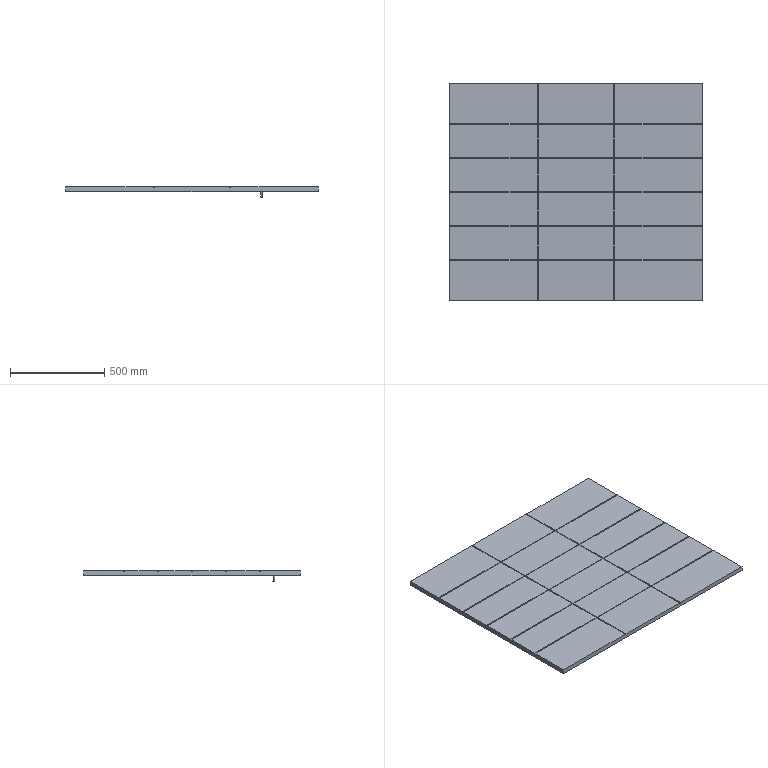Part | SolidWorks | features ICE 3, Extrusion 1, LPattern 1, Sweep 1 | 1 solid | 84 faces | box 1340 x 1150 x 55 mm | volume 38292286 mm3 | plane 80 | cylinder 4 | commonest cylinder face diameters 3 x2 10 x2